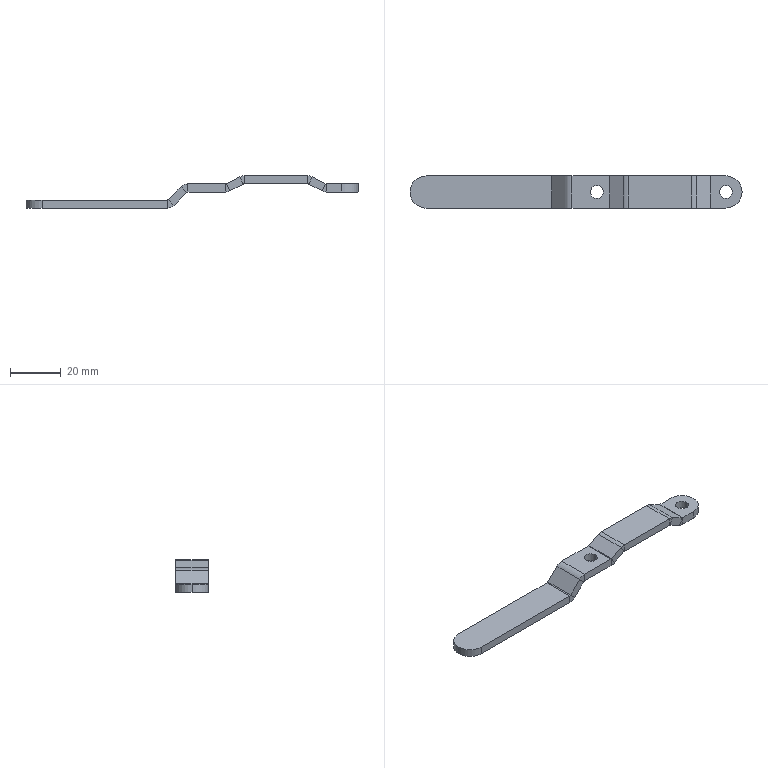Part | SolidWorks | features Fillet 3, Cut 1, Extrusion 1, FlattenBends 1, ProcessBends 1, SheetMetal 1 | 1 solid | 60 faces | box 130.683 x 12.7 x 12.7 mm | volume 5187 mm3 | plane 40 | cylinder 20 | commonest cylinder face diameters 1.27 x6 7.62 x6 5.08 x4 12.7 x4
STEP:
#1=CARTESIAN_POINT('',(-2.35,0.25,0.));
#2=VERTEX_POINT('',#1);
#3=CARTESIAN_POINT('',(-2.15,0.25,0.));
#4=VERTEX_POINT('',#3);
#5=CARTESIAN_POINT('',(-2.25,0.25,0.));
#6=DIRECTION('',(0.,0.,1.));
#7=DIRECTION('',(1.,0.,0.));
#8=AXIS2_PLACEMENT_3D('',#5,#6,#7);
#9=CIRCLE('',#8,0.1);
#10=EDGE_CURVE('',#2,#4,#9,.T.);
#11=ORIENTED_EDGE('',*,*,#10,.F.);
#12=CARTESIAN_POINT('',(-2.35,0.25,0.125));
#13=VERTEX_POINT('',#12);
#14=CARTESIAN_POINT('',(-2.35,0.25,-0.25));
#15=DIRECTION('',(0.,0.,1.));
#16=VECTOR('',#15,39.37);
#17=LINE('',#14,#16);
#18=EDGE_CURVE('',#2,#13,#17,.T.);
#19=ORIENTED_EDGE('',*,*,#18,.T.);
#20=CARTESIAN_POINT('',(-2.15,0.25,0.125));
#21=VERTEX_POINT('',#20);
#22=CARTESIAN_POINT('',(-2.25,0.25,0.125));
#23=DIRECTION('',(0.,0.,1.));
#24=DIRECTION('',(1.,0.,0.));
#25=AXIS2_PLACEMENT_3D('',#22,#23,#24);
#26=CIRCLE('',#25,0.1);
#27=EDGE_CURVE('',#13,#21,#26,.T.);
#28=ORIENTED_EDGE('',*,*,#27,.T.);
#29=CARTESIAN_POINT('',(-2.15,0.25,-0.25));
#30=DIRECTION('',(0.,0.,1.));
#31=VECTOR('',#30,39.37);
#32=LINE('',#29,#31);
#33=EDGE_CURVE('',#4,#21,#32,.T.);
#34=ORIENTED_EDGE('',*,*,#33,.F.);
#35=EDGE_LOOP('',(#11,#19,#28,#34));
#36=FACE_OUTER_BOUND('',#35,.T.);
#37=CARTESIAN_POINT('',(-2.25,0.25,-0.25));
#38=DIRECTION('',(0.,0.,1.));
#39=DIRECTION('',(1.,0.,0.));
#40=AXIS2_PLACEMENT_3D('',#37,#38,#39);
#41=CYLINDRICAL_SURFACE('',#40,0.1);
#42=ADVANCED_FACE('',(#36),#41,.F.);
#43=CARTESIAN_POINT('',(-0.35,0.25,0.));
#44=VERTEX_POINT('',#43);
#45=CARTESIAN_POINT('',(-0.15,0.25,0.));
#46=VERTEX_POINT('',#45);
#47=CARTESIAN_POINT('',(-0.25,0.25,0.));
#48=DIRECTION('',(0.,0.,1.));
#49=DIRECTION('',(1.,0.,0.));
#50=AXIS2_PLACEMENT_3D('',#47,#48,#49);
#51=CIRCLE('',#50,0.1);
#52=EDGE_CURVE('',#44,#46,#51,.T.);
#53=ORIENTED_EDGE('',*,*,#52,.F.);
#54=CARTESIAN_POINT('',(-0.35,0.25,0.125));
#55=VERTEX_POINT('',#54);
#56=CARTESIAN_POINT('',(-0.35,0.25,-0.25));
#57=DIRECTION('',(0.,0.,1.));
#58=VECTOR('',#57,39.37);
#59=LINE('',#56,#58);
#60=EDGE_CURVE('',#44,#55,#59,.T.);
#61=ORIENTED_EDGE('',*,*,#60,.T.);
#62=CARTESIAN_POINT('',(-0.15,0.25,0.125));
#63=VERTEX_POINT('',#62);
#64=CARTESIAN_POINT('',(-0.25,0.25,0.125));
#65=DIRECTION('',(0.,0.,1.));
#66=DIRECTION('',(1.,0.,0.));
#67=AXIS2_PLACEMENT_3D('',#64,#65,#66);
#68=CIRCLE('',#67,0.1);
#69=EDGE_CURVE('',#55,#63,#68,.T.);
#70=ORIENTED_EDGE('',*,*,#69,.T.);
#71=CARTESIAN_POINT('',(-0.15,0.25,-0.25));
#72=DIRECTION('',(0.,0.,1.));
#73=VECTOR('',#72,39.37);
#74=LINE('',#71,#73);
#75=EDGE_CURVE('',#46,#63,#74,.T.);
#76=ORIENTED_EDGE('',*,*,#75,.F.);
#77=EDGE_LOOP('',(#53,#61,#70,#76));
#78=FACE_OUTER_BOUND('',#77,.T.);
#79=CARTESIAN_POINT('',(-0.25,0.25,-0.25));
#80=DIRECTION('',(0.,0.,1.));
#81=DIRECTION('',(1.,0.,0.));
#82=AXIS2_PLACEMENT_3D('',#79,#80,#81);
#83=CYLINDRICAL_SURFACE('',#82,0.1);
#84=ADVANCED_FACE('',(#78),#83,.F.);
#85=CARTESIAN_POINT('',(-0.25,0.25,0.));
#86=DIRECTION('',(0.,0.,1.));
#87=DIRECTION('',(1.,0.,0.));
#88=AXIS2_PLACEMENT_3D('',#85,#86,#87);
#89=CIRCLE('',#88,0.1);
#90=EDGE_CURVE('',#46,#44,#89,.T.);
#91=ORIENTED_EDGE('',*,*,#90,.T.);
#92=ORIENTED_EDGE('',*,*,#52,.T.);
#93=EDGE_LOOP('',(#91,#92));
#94=FACE_BOUND('',#93,.T.);
#95=CARTESIAN_POINT('',(-0.25,0.5,0.));
#96=VERTEX_POINT('',#95);
#97=CARTESIAN_POINT('',(-0.4846,0.5,0.));
#98=VERTEX_POINT('',#97);
#99=CARTESIAN_POINT('',(0.,0.5,0.));
#100=DIRECTION('',(-1.,0.,0.));
#101=VECTOR('',#100,39.37);
#102=LINE('',#99,#101);
#103=EDGE_CURVE('',#96,#98,#102,.T.);
#104=ORIENTED_EDGE('',*,*,#103,.F.);
#105=CARTESIAN_POINT('',(0.,0.25,0.));
#106=VERTEX_POINT('',#105);
#107=CARTESIAN_POINT('',(-0.25,0.25,0.));
#108=DIRECTION('',(0.,0.,-1.));
#109=DIRECTION('',(1.,0.,0.));
#110=AXIS2_PLACEMENT_3D('',#107,#108,#109);
#111=CIRCLE('',#110,0.25);
#112=EDGE_CURVE('',#96,#106,#111,.T.);
#113=ORIENTED_EDGE('',*,*,#112,.T.);
#114=CARTESIAN_POINT('',(-0.25,0.,0.));
#115=VERTEX_POINT('',#114);
#116=CARTESIAN_POINT('',(-0.25,0.25,0.));
#117=DIRECTION('',(0.,0.,-1.));
#118=DIRECTION('',(1.,0.,0.));
#119=AXIS2_PLACEMENT_3D('',#116,#117,#118);
#120=CIRCLE('',#119,0.25);
#121=EDGE_CURVE('',#106,#115,#120,.T.);
#122=ORIENTED_EDGE('',*,*,#121,.T.);
#123=CARTESIAN_POINT('',(-0.4846,0.,0.));
#124=VERTEX_POINT('',#123);
#125=CARTESIAN_POINT('',(0.,0.,0.));
#126=DIRECTION('',(-1.,0.,0.));
#127=VECTOR('',#126,39.37);
#128=LINE('',#125,#127);
#129=EDGE_CURVE('',#115,#124,#128,.T.);
#130=ORIENTED_EDGE('',*,*,#129,.T.);
#131=CARTESIAN_POINT('',(-0.4846,0.5,0.));
#132=DIRECTION('',(0.,1.,0.));
#133=VECTOR('',#132,39.37);
#134=LINE('',#131,#133);
#135=EDGE_CURVE('',#124,#98,#134,.T.);
#136=ORIENTED_EDGE('',*,*,#135,.T.);
#137=EDGE_LOOP('',(#104,#113,#122,#130,#136));
#138=FACE_OUTER_BOUND('',#137,.T.);
#139=CARTESIAN_POINT('',(0.,0.5,0.));
#140=DIRECTION('',(0.,0.,1.));
#141=DIRECTION('',(1.,0.,0.));
#142=AXIS2_PLACEMENT_3D('',#139,#140,#141);
#143=PLANE('',#142);
#144=ADVANCED_FACE('',(#94,#138),#143,.F.);
#145=ORIENTED_EDGE('',*,*,#60,.F.);
#146=ORIENTED_EDGE('',*,*,#90,.F.);
#147=ORIENTED_EDGE('',*,*,#75,.T.);
#148=CARTESIAN_POINT('',(-0.25,0.25,0.125));
#149=DIRECTION('',(0.,0.,1.));
#150=DIRECTION('',(1.,0.,0.));
#151=AXIS2_PLACEMENT_3D('',#148,#149,#150);
#152=CIRCLE('',#151,0.1);
#153=EDGE_CURVE('',#63,#55,#152,.T.);
#154=ORIENTED_EDGE('',*,*,#153,.T.);
#155=EDGE_LOOP('',(#145,#146,#147,#154));
#156=FACE_OUTER_BOUND('',#155,.T.);
#157=CARTESIAN_POINT('',(-0.25,0.25,-0.25));
#158=DIRECTION('',(0.,0.,1.));
#159=DIRECTION('',(1.,0.,0.));
#160=AXIS2_PLACEMENT_3D('',#157,#158,#159);
#161=CYLINDRICAL_SURFACE('',#160,0.1);
#162=ADVANCED_FACE('',(#156),#161,.F.);
#163=ORIENTED_EDGE('',*,*,#153,.F.);
#164=ORIENTED_EDGE('',*,*,#69,.F.);
#165=EDGE_LOOP('',(#163,#164));
#166=FACE_BOUND('',#165,.T.);
#167=CARTESIAN_POINT('',(-0.25,0.,0.125));
#168=VERTEX_POINT('',#167);
#169=CARTESIAN_POINT('',(0.,0.25,0.125));
#170=VERTEX_POINT('',#169);
#171=CARTESIAN_POINT('',(-0.25,0.25,0.125));
#172=DIRECTION('',(0.,0.,1.));
#173=DIRECTION('',(1.,0.,0.));
#174=AXIS2_PLACEMENT_3D('',#171,#172,#173);
#175=CIRCLE('',#174,0.25);
#176=EDGE_CURVE('',#168,#170,#175,.T.);
#177=ORIENTED_EDGE('',*,*,#176,.T.);
#178=CARTESIAN_POINT('',(-0.25,0.5,0.125));
#179=VERTEX_POINT('',#178);
#180=CARTESIAN_POINT('',(-0.25,0.25,0.125));
#181=DIRECTION('',(0.,0.,1.));
#182=DIRECTION('',(1.,0.,0.));
#183=AXIS2_PLACEMENT_3D('',#180,#181,#182);
#184=CIRCLE('',#183,0.25);
#185=EDGE_CURVE('',#170,#179,#184,.T.);
#186=ORIENTED_EDGE('',*,*,#185,.T.);
#187=CARTESIAN_POINT('',(-0.4846,0.5,0.125));
#188=VERTEX_POINT('',#187);
#189=CARTESIAN_POINT('',(0.,0.5,0.125));
#190=DIRECTION('',(-1.,0.,0.));
#191=VECTOR('',#190,39.37);
#192=LINE('',#189,#191);
#193=EDGE_CURVE('',#179,#188,#192,.T.);
#194=ORIENTED_EDGE('',*,*,#193,.T.);
#195=CARTESIAN_POINT('',(-0.4846,0.,0.125));
#196=VERTEX_POINT('',#195);
#197=CARTESIAN_POINT('',(-0.4846,0.,0.125));
#198=DIRECTION('',(0.,-1.,0.));
#199=VECTOR('',#198,39.37);
#200=LINE('',#197,#199);
#201=EDGE_CURVE('',#188,#196,#200,.T.);
#202=ORIENTED_EDGE('',*,*,#201,.T.);
#203=CARTESIAN_POINT('',(0.,0.,0.125));
#204=DIRECTION('',(-1.,0.,0.));
#205=VECTOR('',#204,39.37);
#206=LINE('',#203,#205);
#207=EDGE_CURVE('',#168,#196,#206,.T.);
#208=ORIENTED_EDGE('',*,*,#207,.F.);
#209=EDGE_LOOP('',(#177,#186,#194,#202,#208));
#210=FACE_OUTER_BOUND('',#209,.T.);
#211=CARTESIAN_POINT('',(0.,0.5,0.125));
#212=DIRECTION('',(0.,0.,1.));
#213=DIRECTION('',(1.,0.,0.));
#214=AXIS2_PLACEMENT_3D('',#211,#212,#213);
#215=PLANE('',#214);
#216=ADVANCED_FACE('',(#166,#210),#215,.T.);
#217=CARTESIAN_POINT('',(-0.25,0.,1.518));
#218=DIRECTION('',(0.,0.,-1.));
#219=VECTOR('',#218,39.37);
#220=LINE('',#217,#219);
#221=EDGE_CURVE('',#168,#115,#220,.T.);
#222=ORIENTED_EDGE('',*,*,#221,.T.);
#223=ORIENTED_EDGE('',*,*,#121,.F.);
#224=CARTESIAN_POINT('',(0.,0.25,1.518));
#225=DIRECTION('',(0.,0.,-1.));
#226=VECTOR('',#225,39.37);
#227=LINE('',#224,#226);
#228=EDGE_CURVE('',#170,#106,#227,.T.);
#229=ORIENTED_EDGE('',*,*,#228,.F.);
#230=ORIENTED_EDGE('',*,*,#176,.F.);
#231=EDGE_LOOP('',(#222,#223,#229,#230));
#232=FACE_OUTER_BOUND('',#231,.T.);
#233=CARTESIAN_POINT('',(-0.25,0.25,1.518));
#234=DIRECTION('',(0.,0.,-1.));
#235=DIRECTION('',(-1.,0.,0.));
#236=AXIS2_PLACEMENT_3D('',#233,#234,#235);
#237=CYLINDRICAL_SURFACE('',#236,0.25);
#238=ADVANCED_FACE('',(#232),#237,.T.);
#239=ORIENTED_EDGE('',*,*,#228,.T.);
#240=ORIENTED_EDGE('',*,*,#112,.F.);
#241=CARTESIAN_POINT('',(-0.25,0.5,1.518));
#242=DIRECTION('',(0.,0.,-1.));
#243=VECTOR('',#242,39.37);
#244=LINE('',#241,#243);
#245=EDGE_CURVE('',#179,#96,#244,.T.);
#246=ORIENTED_EDGE('',*,*,#245,.F.);
#247=ORIENTED_EDGE('',*,*,#185,.F.);
#248=EDGE_LOOP('',(#239,#240,#246,#247));
#249=FACE_OUTER_BOUND('',#248,.T.);
#250=CARTESIAN_POINT('',(-0.25,0.25,1.518));
#251=DIRECTION('',(0.,0.,-1.));
#252=DIRECTION('',(-1.,0.,0.));
#253=AXIS2_PLACEMENT_3D('',#250,#251,#252);
#254=CYLINDRICAL_SURFACE('',#253,0.25);
#255=ADVANCED_FACE('',(#249),#254,.T.);
#256=ORIENTED_EDGE('',*,*,#245,.T.);
#257=ORIENTED_EDGE('',*,*,#103,.T.);
#258=CARTESIAN_POINT('',(-0.4846,0.5,1.518));
#259=DIRECTION('',(0.,0.,-1.));
#260=VECTOR('',#259,39.37);
#261=LINE('',#258,#260);
#262=EDGE_CURVE('',#188,#98,#261,.T.);
#263=ORIENTED_EDGE('',*,*,#262,.F.);
#264=ORIENTED_EDGE('',*,*,#193,.F.);
#265=EDGE_LOOP('',(#256,#257,#263,#264));
#266=FACE_OUTER_BOUND('',#265,.T.);
#267=CARTESIAN_POINT('',(0.,0.5,1.518));
#268=DIRECTION('',(0.,-1.,0.));
#269=DIRECTION('',(0.,0.,-1.));
#270=AXIS2_PLACEMENT_3D('',#267,#268,#269);
#271=PLANE('',#270);
#272=ADVANCED_FACE('',(#266),#271,.F.);
#273=ORIENTED_EDGE('',*,*,#129,.F.);
#274=ORIENTED_EDGE('',*,*,#221,.F.);
#275=ORIENTED_EDGE('',*,*,#207,.T.);
#276=CARTESIAN_POINT('',(-0.4846,0.,1.518));
#277=DIRECTION('',(0.,0.,-1.));
#278=VECTOR('',#277,39.37);
#279=LINE('',#276,#278);
#280=EDGE_CURVE('',#196,#124,#279,.T.);
#281=ORIENTED_EDGE('',*,*,#280,.T.);
#282=EDGE_LOOP('',(#273,#274,#275,#281));
#283=FACE_OUTER_BOUND('',#282,.T.);
#284=CARTESIAN_POINT('',(0.,0.,1.518));
#285=DIRECTION('',(0.,-1.,0.));
#286=DIRECTION('',(0.,0.,-1.));
#287=AXIS2_PLACEMENT_3D('',#284,#285,#286);
#288=PLANE('',#287);
#289=ADVANCED_FACE('',(#283),#288,.T.);
#290=CARTESIAN_POINT('',(-0.7647,0.5,0.1224));
#291=VERTEX_POINT('',#290);
#292=CARTESIAN_POINT('',(-0.7088,0.5,0.2342));
#293=VERTEX_POINT('',#292);
#294=CARTESIAN_POINT('',(-1.204,0.5,-0.7566));
#295=DIRECTION('',(0.4472,0.,0.8944));
#296=VECTOR('',#295,39.37);
#297=LINE('',#294,#296);
#298=EDGE_CURVE('',#291,#293,#297,.T.);
#299=ORIENTED_EDGE('',*,*,#298,.T.);
#300=CARTESIAN_POINT('',(-0.4958,0.5,0.1276));
#301=VERTEX_POINT('',#300);
#302=CARTESIAN_POINT('',(-0.4905,0.5,0.125));
#303=DIRECTION('',(-0.8944,0.,0.4472));
#304=VECTOR('',#303,39.37);
#305=LINE('',#302,#304);
#306=EDGE_CURVE('',#301,#293,#305,.T.);
#307=ORIENTED_EDGE('',*,*,#306,.F.);
#308=CARTESIAN_POINT('',(-0.5517,0.5,0.01584));
#309=VERTEX_POINT('',#308);
#310=CARTESIAN_POINT('',(-0.9911,0.5,-0.8631));
#311=DIRECTION('',(0.4472,0.,0.8944));
#312=VECTOR('',#311,39.37);
#313=LINE('',#310,#312);
#314=EDGE_CURVE('',#309,#301,#313,.T.);
#315=ORIENTED_EDGE('',*,*,#314,.F.);
#316=CARTESIAN_POINT('',(-0.52,0.5,0.));
#317=DIRECTION('',(-0.8944,0.,0.4472));
#318=VECTOR('',#317,39.37);
#319=LINE('',#316,#318);
#320=EDGE_CURVE('',#309,#291,#319,.T.);
#321=ORIENTED_EDGE('',*,*,#320,.T.);
#322=EDGE_LOOP('',(#299,#307,#315,#321));
#323=FACE_OUTER_BOUND('',#322,.T.);
#324=CARTESIAN_POINT('',(-0.9595,0.5,-0.8789));
#325=DIRECTION('',(0.,1.,0.));
#326=DIRECTION('',(0.4472,0.,0.8944));
#327=AXIS2_PLACEMENT_3D('',#324,#325,#326);
#328=PLANE('',#327);
#329=ADVANCED_FACE('',(#323),#328,.T.);
#330=CARTESIAN_POINT('',(-0.4958,0.,0.1276));
#331=VERTEX_POINT('',#330);
#332=CARTESIAN_POINT('',(-0.7088,0.,0.2342));
#333=VERTEX_POINT('',#332);
#334=CARTESIAN_POINT('',(-0.4905,0.,0.125));
#335=DIRECTION('',(-0.8944,0.,0.4472));
#336=VECTOR('',#335,39.37);
#337=LINE('',#334,#336);
#338=EDGE_CURVE('',#331,#333,#337,.T.);
#339=ORIENTED_EDGE('',*,*,#338,.T.);
#340=CARTESIAN_POINT('',(-0.7647,0.,0.1224));
#341=VERTEX_POINT('',#340);
#342=CARTESIAN_POINT('',(-1.204,0.,-0.7566));
#343=DIRECTION('',(0.4472,0.,0.8944));
#344=VECTOR('',#343,39.37);
#345=LINE('',#342,#344);
#346=EDGE_CURVE('',#341,#333,#345,.T.);
#347=ORIENTED_EDGE('',*,*,#346,.F.);
#348=CARTESIAN_POINT('',(-0.5517,0.,0.01584));
#349=VERTEX_POINT('',#348);
#350=CARTESIAN_POINT('',(-0.52,0.,0.));
#351=DIRECTION('',(-0.8944,0.,0.4472));
#352=VECTOR('',#351,39.37);
#353=LINE('',#350,#352);
#354=EDGE_CURVE('',#349,#341,#353,.T.);
#355=ORIENTED_EDGE('',*,*,#354,.F.);
#356=CARTESIAN_POINT('',(-0.9911,0.,-0.8631));
#357=DIRECTION('',(0.4472,0.,0.8944));
#358=VECTOR('',#357,39.37);
#359=LINE('',#356,#358);
#360=EDGE_CURVE('',#349,#331,#359,.T.);
#361=ORIENTED_EDGE('',*,*,#360,.T.);
#362=EDGE_LOOP('',(#339,#347,#355,#361));
#363=FACE_OUTER_BOUND('',#362,.T.);
#364=CARTESIAN_POINT('',(-0.9595,0.,-0.8789));
#365=DIRECTION('',(0.,1.,0.));
#366=DIRECTION('',(0.4472,0.,0.8944));
#367=AXIS2_PLACEMENT_3D('',#364,#365,#366);
#368=PLANE('',#367);
#369=ADVANCED_FACE('',(#363),#368,.F.);
#370=ORIENTED_EDGE('',*,*,#320,.F.);
#371=CARTESIAN_POINT('',(-0.5517,0.5,0.01584));
#372=DIRECTION('',(0.,-1.,0.));
#373=VECTOR('',#372,39.37);
#374=LINE('',#371,#373);
#375=EDGE_CURVE('',#309,#349,#374,.T.);
#376=ORIENTED_EDGE('',*,*,#375,.T.);
#377=ORIENTED_EDGE('',*,*,#354,.T.);
#378=CARTESIAN_POINT('',(-0.7647,0.5,0.1224));
#379=DIRECTION('',(0.,1.,0.));
#380=VECTOR('',#379,39.37);
#381=LINE('',#378,#380);
#382=EDGE_CURVE('',#341,#291,#381,.T.);
#383=ORIENTED_EDGE('',*,*,#382,.T.);
#384=EDGE_LOOP('',(#370,#376,#377,#383));
#385=FACE_OUTER_BOUND('',#384,.T.);
#386=CARTESIAN_POINT('',(-0.52,0.5,0.));
#387=DIRECTION('',(0.4472,0.,0.8944));
#388=DIRECTION('',(0.8944,0.,-0.4472));
#389=AXIS2_PLACEMENT_3D('',#386,#387,#388);
#390=PLANE('',#389);
#391=ADVANCED_FACE('',(#385),#390,.F.);
#392=ORIENTED_EDGE('',*,*,#306,.T.);
#393=CARTESIAN_POINT('',(-0.7088,0.5,0.2342));
#394=DIRECTION('',(0.,-1.,0.));
#395=VECTOR('',#394,39.37);
#396=LINE('',#393,#395);
#397=EDGE_CURVE('',#293,#333,#396,.T.);
#398=ORIENTED_EDGE('',*,*,#397,.T.);
#399=ORIENTED_EDGE('',*,*,#338,.F.);
#400=CARTESIAN_POINT('',(-0.4958,0.5,0.1276));
#401=DIRECTION('',(0.,1.,0.));
#402=VECTOR('',#401,39.37);
#403=LINE('',#400,#402);
#404=EDGE_CURVE('',#331,#301,#403,.T.);
#405=ORIENTED_EDGE('',*,*,#404,.T.);
#406=EDGE_LOOP('',(#392,#398,#399,#405));
#407=FACE_OUTER_BOUND('',#406,.T.);
#408=CARTESIAN_POINT('',(-0.4905,0.5,0.125));
#409=DIRECTION('',(0.4472,0.,0.8944));
#410=DIRECTION('',(0.8944,0.,-0.4472));
#411=AXIS2_PLACEMENT_3D('',#408,#409,#410);
#412=PLANE('',#411);
#413=ADVANCED_FACE('',(#407),#412,.T.);
#414=CARTESIAN_POINT('',(-0.7759,0.,0.25));
#415=VERTEX_POINT('',#414);
#416=CARTESIAN_POINT('',(-1.764,0.,0.25));
#417=VERTEX_POINT('',#416);
#418=CARTESIAN_POINT('',(-0.7405,0.,0.25));
#419=DIRECTION('',(-1.,0.,0.));
#420=VECTOR('',#419,39.37);
#421=LINE('',#418,#420);
#422=EDGE_CURVE('',#415,#417,#421,.T.);
#423=ORIENTED_EDGE('',*,*,#422,.T.);
#424=CARTESIAN_POINT('',(-1.764,0.,0.125));
#425=VERTEX_POINT('',#424);
#426=CARTESIAN_POINT('',(-1.764,0.,-1.965));
#427=DIRECTION('',(0.,0.,1.));
#428=VECTOR('',#427,39.37);
#429=LINE('',#426,#428);
#430=EDGE_CURVE('',#425,#417,#429,.T.);
#431=ORIENTED_EDGE('',*,*,#430,.F.);
#432=CARTESIAN_POINT('',(-0.7759,0.,0.125));
#433=VERTEX_POINT('',#432);
#434=CARTESIAN_POINT('',(-0.77,0.,0.125));
#435=DIRECTION('',(-1.,0.,0.));
#436=VECTOR('',#435,39.37);
#437=LINE('',#434,#436);
#438=EDGE_CURVE('',#433,#425,#437,.T.);
#439=ORIENTED_EDGE('',*,*,#438,.F.);
#440=CARTESIAN_POINT('',(-0.7759,0.,-1.965));
#441=DIRECTION('',(0.,0.,1.));
#442=VECTOR('',#441,39.37);
#443=LINE('',#440,#442);
#444=EDGE_CURVE('',#433,#415,#443,.T.);
#445=ORIENTED_EDGE('',*,*,#444,.T.);
#446=EDGE_LOOP('',(#423,#431,#439,#445));
#447=FACE_OUTER_BOUND('',#446,.T.);
#448=CARTESIAN_POINT('',(-0.77,0.,-1.965));
#449=DIRECTION('',(0.,1.,0.));
#450=DIRECTION('',(0.,0.,1.));
#451=AXIS2_PLACEMENT_3D('',#448,#449,#450);
#452=PLANE('',#451);
#453=ADVANCED_FACE('',(#447),#452,.F.);
#454=CARTESIAN_POINT('',(-1.764,0.5,0.125));
#455=VERTEX_POINT('',#454);
#456=CARTESIAN_POINT('',(-1.764,0.5,0.25));
#457=VERTEX_POINT('',#456);
#458=CARTESIAN_POINT('',(-1.764,0.5,-1.965));
#459=DIRECTION('',(0.,0.,1.));
#460=VECTOR('',#459,39.37);
#461=LINE('',#458,#460);
#462=EDGE_CURVE('',#455,#457,#461,.T.);
#463=ORIENTED_EDGE('',*,*,#462,.T.);
#464=CARTESIAN_POINT('',(-0.7759,0.5,0.25));
#465=VERTEX_POINT('',#464);
#466=CARTESIAN_POINT('',(-0.7405,0.5,0.25));
#467=DIRECTION('',(-1.,0.,0.));
#468=VECTOR('',#467,39.37);
#469=LINE('',#466,#468);
#470=EDGE_CURVE('',#465,#457,#469,.T.);
#471=ORIENTED_EDGE('',*,*,#470,.F.);
#472=CARTESIAN_POINT('',(-0.7759,0.5,0.125));
#473=VERTEX_POINT('',#472);
#474=CARTESIAN_POINT('',(-0.7759,0.5,-1.965));
#475=DIRECTION('',(0.,0.,1.));
#476=VECTOR('',#475,39.37);
#477=LINE('',#474,#476);
#478=EDGE_CURVE('',#473,#465,#477,.T.);
#479=ORIENTED_EDGE('',*,*,#478,.F.);
#480=CARTESIAN_POINT('',(-0.77,0.5,0.125));
#481=DIRECTION('',(-1.,0.,0.));
#482=VECTOR('',#481,39.37);
#483=LINE('',#480,#482);
#484=EDGE_CURVE('',#473,#455,#483,.T.);
#485=ORIENTED_EDGE('',*,*,#484,.T.);
#486=EDGE_LOOP('',(#463,#471,#479,#485));
#487=FACE_OUTER_BOUND('',#486,.T.);
#488=CARTESIAN_POINT('',(-0.77,0.5,-1.965));
#489=DIRECTION('',(0.,1.,0.));
#490=DIRECTION('',(0.,0.,1.));
#491=AXIS2_PLACEMENT_3D('',#488,#489,#490);
#492=PLANE('',#491);
#493=ADVANCED_FACE('',(#487),#492,.T.);
#494=ORIENTED_EDGE('',*,*,#438,.T.);
#495=CARTESIAN_POINT('',(-1.764,0.5,0.125));
#496=DIRECTION('',(0.,1.,0.));
#497=VECTOR('',#496,39.37);
#498=LINE('',#495,#497);
#499=EDGE_CURVE('',#425,#455,#498,.T.);
#500=ORIENTED_EDGE('',*,*,#499,.T.);
#501=ORIENTED_EDGE('',*,*,#484,.F.);
#502=CARTESIAN_POINT('',(-0.7759,0.,0.125));
#503=DIRECTION('',(0.,-1.,0.));
#504=VECTOR('',#503,39.37);
#505=LINE('',#502,#504);
#506=EDGE_CURVE('',#473,#433,#505,.T.);
#507=ORIENTED_EDGE('',*,*,#506,.T.);
#508=EDGE_LOOP('',(#494,#500,#501,#507));
#509=FACE_OUTER_BOUND('',#508,.T.);
#510=CARTESIAN_POINT('',(-0.77,0.5,0.125));
#511=DIRECTION('',(0.,0.,1.));
#512=DIRECTION('',(1.,0.,0.));
#513=AXIS2_PLACEMENT_3D('',#510,#511,#512);
#514=PLANE('',#513);
#515=ADVANCED_FACE('',(#509),#514,.F.);
#516=ORIENTED_EDGE('',*,*,#470,.T.);
#517=CARTESIAN_POINT('',(-1.764,0.5,0.25));
#518=DIRECTION('',(0.,-1.,0.));
#519=VECTOR('',#518,39.37);
#520=LINE('',#517,#519);
#521=EDGE_CURVE('',#457,#417,#520,.T.);
#522=ORIENTED_EDGE('',*,*,#521,.T.);
#523=ORIENTED_EDGE('',*,*,#422,.F.);
#524=CARTESIAN_POINT('',(-0.7759,0.5,0.25));
#525=DIRECTION('',(0.,1.,0.));
#526=VECTOR('',#525,39.37);
#527=LINE('',#524,#526);
#528=EDGE_CURVE('',#415,#465,#527,.T.);
#529=ORIENTED_EDGE('',*,*,#528,.T.);
#530=EDGE_LOOP('',(#516,#522,#523,#529));
#531=FACE_OUTER_BOUND('',#530,.T.);
#532=CARTESIAN_POINT('',(-0.7405,0.5,0.25));
#533=DIRECTION('',(0.,0.,1.));
#534=DIRECTION('',(1.,0.,0.));
#535=AXIS2_PLACEMENT_3D('',#532,#533,#534);
#536=PLANE('',#535);
#537=ADVANCED_FACE('',(#531),#536,.T.);
#538=CARTESIAN_POINT('',(-1.775,0.,0.1224));
#539=VERTEX_POINT('',#538);
#540=CARTESIAN_POINT('',(-1.988,0.,0.01584));
#541=VERTEX_POINT('',#540);
#542=CARTESIAN_POINT('',(-1.77,0.,0.125));
#543=DIRECTION('',(-0.8944,0.,-0.4472));
#544=VECTOR('',#543,39.37);
#545=LINE('',#542,#544);
#546=EDGE_CURVE('',#539,#541,#545,.T.);
#547=ORIENTED_EDGE('',*,*,#546,.T.);
#548=CARTESIAN_POINT('',(-1.988,0.5,0.01584));
#549=VERTEX_POINT('',#548);
#550=CARTESIAN_POINT('',(-1.988,0.5,0.01584));
#551=DIRECTION('',(0.,1.,0.));
#552=VECTOR('',#551,39.37);
#553=LINE('',#550,#552);
#554=EDGE_CURVE('',#541,#549,#553,.T.);
#555=ORIENTED_EDGE('',*,*,#554,.T.);
#556=CARTESIAN_POINT('',(-1.775,0.5,0.1224));
#557=VERTEX_POINT('',#556);
#558=CARTESIAN_POINT('',(-1.77,0.5,0.125));
#559=DIRECTION('',(-0.8944,0.,-0.4472));
#560=VECTOR('',#559,39.37);
#561=LINE('',#558,#560);
#562=EDGE_CURVE('',#557,#549,#561,.T.);
#563=ORIENTED_EDGE('',*,*,#562,.F.);
#564=CARTESIAN_POINT('',(-1.775,0.,0.1224));
#565=DIRECTION('',(0.,-1.,0.));
#566=VECTOR('',#565,39.37);
#567=LINE('',#564,#566);
#568=EDGE_CURVE('',#557,#539,#567,.T.);
#569=ORIENTED_EDGE('',*,*,#568,.T.);
#570=EDGE_LOOP('',(#547,#555,#563,#569));
#571=FACE_OUTER_BOUND('',#570,.T.);
#572=CARTESIAN_POINT('',(-1.77,0.5,0.125));
#573=DIRECTION('',(-0.4472,0.,0.8944));
#574=DIRECTION('',(0.8944,0.,0.4472));
#575=AXIS2_PLACEMENT_3D('',#572,#573,#574);
#576=PLANE('',#575);
#577=ADVANCED_FACE('',(#571),#576,.F.);
#578=ORIENTED_EDGE('',*,*,#546,.F.);
#579=CARTESIAN_POINT('',(-1.831,0.,0.2342));
#580=VERTEX_POINT('',#579);
#581=CARTESIAN_POINT('',(-2.327,0.,1.225));
#582=DIRECTION('',(0.4472,0.,-0.8944));
#583=VECTOR('',#582,39.37);
#584=LINE('',#581,#583);
#585=EDGE_CURVE('',#580,#539,#584,.T.);
#586=ORIENTED_EDGE('',*,*,#585,.F.);
#587=CARTESIAN_POINT('',(-2.044,0.,0.1276));
#588=VERTEX_POINT('',#587);
#589=CARTESIAN_POINT('',(-1.8,0.,0.25));
#590=DIRECTION('',(-0.8944,0.,-0.4472));
#591=VECTOR('',#590,39.37);
#592=LINE('',#589,#591);
#593=EDGE_CURVE('',#580,#588,#592,.T.);
#594=ORIENTED_EDGE('',*,*,#593,.T.);
#595=CARTESIAN_POINT('',(-2.54,0.,1.118));
#596=DIRECTION('',(0.4472,0.,-0.8944));
#597=VECTOR('',#596,39.37);
#598=LINE('',#595,#597);
#599=EDGE_CURVE('',#588,#541,#598,.T.);
#600=ORIENTED_EDGE('',*,*,#599,.T.);
#601=EDGE_LOOP('',(#578,#586,#594,#600));
#602=FACE_OUTER_BOUND('',#601,.T.);
#603=CARTESIAN_POINT('',(-2.295,0.,1.241));
#604=DIRECTION('',(0.,-1.,0.));
#605=DIRECTION('',(0.4472,0.,-0.8944));
#606=AXIS2_PLACEMENT_3D('',#603,#604,#605);
#607=PLANE('',#606);
#608=ADVANCED_FACE('',(#602),#607,.T.);
#609=CARTESIAN_POINT('',(-1.831,0.5,0.2342));
#610=VERTEX_POINT('',#609);
#611=CARTESIAN_POINT('',(-2.327,0.5,1.225));
#612=DIRECTION('',(0.4472,0.,-0.8944));
#613=VECTOR('',#612,39.37);
#614=LINE('',#611,#613);
#615=EDGE_CURVE('',#610,#557,#614,.T.);
#616=ORIENTED_EDGE('',*,*,#615,.T.);
#617=ORIENTED_EDGE('',*,*,#562,.T.);
#618=CARTESIAN_POINT('',(-2.044,0.5,0.1276));
#619=VERTEX_POINT('',#618);
#620=CARTESIAN_POINT('',(-2.54,0.5,1.118));
#621=DIRECTION('',(0.4472,0.,-0.8944));
#622=VECTOR('',#621,39.37);
#623=LINE('',#620,#622);
#624=EDGE_CURVE('',#619,#549,#623,.T.);
#625=ORIENTED_EDGE('',*,*,#624,.F.);
#626=CARTESIAN_POINT('',(-1.8,0.5,0.25));
#627=DIRECTION('',(-0.8944,0.,-0.4472));
#628=VECTOR('',#627,39.37);
#629=LINE('',#626,#628);
#630=EDGE_CURVE('',#610,#619,#629,.T.);
#631=ORIENTED_EDGE('',*,*,#630,.F.);
#632=EDGE_LOOP('',(#616,#617,#625,#631));
#633=FACE_OUTER_BOUND('',#632,.T.);
#634=CARTESIAN_POINT('',(-2.295,0.5,1.241));
#635=DIRECTION('',(0.,-1.,0.));
#636=DIRECTION('',(0.4472,0.,-0.8944));
#637=AXIS2_PLACEMENT_3D('',#634,#635,#636);
#638=PLANE('',#637);
#639=ADVANCED_FACE('',(#633),#638,.F.);
#640=ORIENTED_EDGE('',*,*,#593,.F.);
#641=CARTESIAN_POINT('',(-1.831,0.5,0.2342));
#642=DIRECTION('',(0.,1.,0.));
#643=VECTOR('',#642,39.37);
#644=LINE('',#641,#643);
#645=EDGE_CURVE('',#580,#610,#644,.T.);
#646=ORIENTED_EDGE('',*,*,#645,.T.);
#647=ORIENTED_EDGE('',*,*,#630,.T.);
#648=CARTESIAN_POINT('',(-2.044,0.,0.1276));
#649=DIRECTION('',(0.,-1.,0.));
#650=VECTOR('',#649,39.37);
#651=LINE('',#648,#650);
#652=EDGE_CURVE('',#619,#588,#651,.T.);
#653=ORIENTED_EDGE('',*,*,#652,.T.);
#654=EDGE_LOOP('',(#640,#646,#647,#653));
#655=FACE_OUTER_BOUND('',#654,.T.);
#656=CARTESIAN_POINT('',(-1.8,0.5,0.25));
#657=DIRECTION('',(-0.4472,0.,0.8944));
#658=DIRECTION('',(0.8944,0.,0.4472));
#659=AXIS2_PLACEMENT_3D('',#656,#657,#658);
#660=PLANE('',#659);
#661=ADVANCED_FACE('',(#655),#660,.T.);
#662=CARTESIAN_POINT('',(-2.25,0.25,0.125));
#663=DIRECTION('',(0.,0.,1.));
#664=DIRECTION('',(1.,0.,0.));
#665=AXIS2_PLACEMENT_3D('',#662,#663,#664);
#666=CIRCLE('',#665,0.1);
#667=EDGE_CURVE('',#21,#13,#666,.T.);
#668=ORIENTED_EDGE('',*,*,#667,.F.);
#669=ORIENTED_EDGE('',*,*,#27,.F.);
#670=EDGE_LOOP('',(#668,#669));
#671=FACE_BOUND('',#670,.T.);
#672=CARTESIAN_POINT('',(-2.055,0.5,0.125));
#673=VERTEX_POINT('',#672);
#674=CARTESIAN_POINT('',(-2.635,0.5,0.125));
#675=VERTEX_POINT('',#674);
#676=CARTESIAN_POINT('',(-2.05,0.5,0.125));
#677=DIRECTION('',(-1.,0.,0.));
#678=VECTOR('',#677,39.37);
#679=LINE('',#676,#678);
#680=EDGE_CURVE('',#673,#675,#679,.T.);
#681=ORIENTED_EDGE('',*,*,#680,.T.);
#682=CARTESIAN_POINT('',(-2.635,0.,0.125));
#683=VERTEX_POINT('',#682);
#684=CARTESIAN_POINT('',(-2.635,0.5,0.125));
#685=DIRECTION('',(0.,-1.,0.));
#686=VECTOR('',#685,39.37);
#687=LINE('',#684,#686);
#688=EDGE_CURVE('',#675,#683,#687,.T.);
#689=ORIENTED_EDGE('',*,*,#688,.T.);
#690=CARTESIAN_POINT('',(-2.055,0.,0.125));
#691=VERTEX_POINT('',#690);
#692=CARTESIAN_POINT('',(-2.05,0.,0.125));
#693=DIRECTION('',(-1.,0.,0.));
#694=VECTOR('',#693,39.37);
#695=LINE('',#692,#694);
#696=EDGE_CURVE('',#691,#683,#695,.T.);
#697=ORIENTED_EDGE('',*,*,#696,.F.);
#698=CARTESIAN_POINT('',(-2.055,0.5,0.125));
#699=DIRECTION('',(0.,1.,0.));
#700=VECTOR('',#699,39.37);
#701=LINE('',#698,#700);
#702=EDGE_CURVE('',#691,#673,#701,.T.);
#703=ORIENTED_EDGE('',*,*,#702,.T.);
#704=EDGE_LOOP('',(#681,#689,#697,#703));
#705=FACE_OUTER_BOUND('',#704,.T.);
#706=CARTESIAN_POINT('',(-2.05,0.5,0.125));
#707=DIRECTION('',(0.,0.,1.));
#708=DIRECTION('',(1.,0.,0.));
#709=AXIS2_PLACEMENT_3D('',#706,#707,#708);
#710=PLANE('',#709);
#711=ADVANCED_FACE('',(#671,#705),#710,.T.);
#712=ORIENTED_EDGE('',*,*,#18,.F.);
#713=CARTESIAN_POINT('',(-2.25,0.25,0.));
#714=DIRECTION('',(0.,0.,1.));
#715=DIRECTION('',(1.,0.,0.));
#716=AXIS2_PLACEMENT_3D('',#713,#714,#715);
#717=CIRCLE('',#716,0.1);
#718=EDGE_CURVE('',#4,#2,#717,.T.);
#719=ORIENTED_EDGE('',*,*,#718,.F.);
#720=ORIENTED_EDGE('',*,*,#33,.T.);
#721=ORIENTED_EDGE('',*,*,#667,.T.);
#722=EDGE_LOOP('',(#712,#719,#720,#721));
#723=FACE_OUTER_BOUND('',#722,.T.);
#724=CARTESIAN_POINT('',(-2.25,0.25,-0.25));
#725=DIRECTION('',(0.,0.,1.));
#726=DIRECTION('',(1.,0.,0.));
#727=AXIS2_PLACEMENT_3D('',#724,#725,#726);
#728=CYLINDRICAL_SURFACE('',#727,0.1);
#729=ADVANCED_FACE('',(#723),#728,.F.);
#730=ORIENTED_EDGE('',*,*,#718,.T.);
#731=ORIENTED_EDGE('',*,*,#10,.T.);
#732=EDGE_LOOP('',(#730,#731));
#733=FACE_BOUND('',#732,.T.);
#734=CARTESIAN_POINT('',(-2.055,0.5,0.));
#735=VERTEX_POINT('',#734);
#736=CARTESIAN_POINT('',(-2.635,0.5,0.));
#737=VERTEX_POINT('',#736);
#738=CARTESIAN_POINT('',(-2.02,0.5,0.));
#739=DIRECTION('',(-1.,0.,0.));
#740=VECTOR('',#739,39.37);
#741=LINE('',#738,#740);
#742=EDGE_CURVE('',#735,#737,#741,.T.);
#743=ORIENTED_EDGE('',*,*,#742,.F.);
#744=CARTESIAN_POINT('',(-2.055,0.,0.));
#745=VERTEX_POINT('',#744);
#746=CARTESIAN_POINT('',(-2.055,0.5,0.));
#747=DIRECTION('',(0.,-1.,0.));
#748=VECTOR('',#747,39.37);
#749=LINE('',#746,#748);
#750=EDGE_CURVE('',#735,#745,#749,.T.);
#751=ORIENTED_EDGE('',*,*,#750,.T.);
#752=CARTESIAN_POINT('',(-2.635,0.,0.));
#753=VERTEX_POINT('',#752);
#754=CARTESIAN_POINT('',(-2.02,0.,0.));
#755=DIRECTION('',(-1.,0.,0.));
#756=VECTOR('',#755,39.37);
#757=LINE('',#754,#756);
#758=EDGE_CURVE('',#745,#753,#757,.T.);
#759=ORIENTED_EDGE('',*,*,#758,.T.);
#760=CARTESIAN_POINT('',(-2.635,0.5,0.));
#761=DIRECTION('',(0.,1.,0.));
#762=VECTOR('',#761,39.37);
#763=LINE('',#760,#762);
#764=EDGE_CURVE('',#753,#737,#763,.T.);
#765=ORIENTED_EDGE('',*,*,#764,.T.);
#766=EDGE_LOOP('',(#743,#751,#759,#765));
#767=FACE_OUTER_BOUND('',#766,.T.);
#768=CARTESIAN_POINT('',(-2.02,0.5,0.));
#769=DIRECTION('',(0.,0.,1.));
#770=DIRECTION('',(1.,0.,0.));
#771=AXIS2_PLACEMENT_3D('',#768,#769,#770);
#772=PLANE('',#771);
#773=ADVANCED_FACE('',(#733,#767),#772,.F.);
#774=CARTESIAN_POINT('',(-2.635,0.5,-1.405));
#775=DIRECTION('',(0.,0.,1.));
#776=VECTOR('',#775,39.37);
#777=LINE('',#774,#776);
#778=EDGE_CURVE('',#737,#675,#777,.T.);
#779=ORIENTED_EDGE('',*,*,#778,.T.);
#780=ORIENTED_EDGE('',*,*,#680,.F.);
#781=CARTESIAN_POINT('',(-2.055,0.5,-1.405));
#782=DIRECTION('',(0.,0.,1.));
#783=VECTOR('',#782,39.37);
#784=LINE('',#781,#783);
#785=EDGE_CURVE('',#735,#673,#784,.T.);
#786=ORIENTED_EDGE('',*,*,#785,.F.);
#787=ORIENTED_EDGE('',*,*,#742,.T.);
#788=EDGE_LOOP('',(#779,#780,#786,#787));
#789=FACE_OUTER_BOUND('',#788,.T.);
#790=CARTESIAN_POINT('',(-2.02,0.5,-1.405));
#791=DIRECTION('',(0.,1.,0.));
#792=DIRECTION('',(0.,0.,1.));
#793=AXIS2_PLACEMENT_3D('',#790,#791,#792);
#794=PLANE('',#793);
#795=ADVANCED_FACE('',(#789),#794,.T.);
#796=ORIENTED_EDGE('',*,*,#696,.T.);
#797=CARTESIAN_POINT('',(-2.635,0.,-1.405));
#798=DIRECTION('',(0.,0.,1.));
#799=VECTOR('',#798,39.37);
#800=LINE('',#797,#799);
#801=EDGE_CURVE('',#753,#683,#800,.T.);
#802=ORIENTED_EDGE('',*,*,#801,.F.);
#803=ORIENTED_EDGE('',*,*,#758,.F.);
#804=CARTESIAN_POINT('',(-2.055,0.,-1.405));
#805=DIRECTION('',(0.,0.,1.));
#806=VECTOR('',#805,39.37);
#807=LINE('',#804,#806);
#808=EDGE_CURVE('',#745,#691,#807,.T.);
#809=ORIENTED_EDGE('',*,*,#808,.T.);
#810=EDGE_LOOP('',(#796,#802,#803,#809));
#811=FACE_OUTER_BOUND('',#810,.T.);
#812=CARTESIAN_POINT('',(-2.02,0.,-1.405));
#813=DIRECTION('',(0.,1.,0.));
#814=DIRECTION('',(0.,0.,1.));
#815=AXIS2_PLACEMENT_3D('',#812,#813,#814);
#816=PLANE('',#815);
#817=ADVANCED_FACE('',(#811),#816,.F.);
#818=CARTESIAN_POINT('',(-2.652,0.,-0.007322));
#819=VERTEX_POINT('',#818);
#820=CARTESIAN_POINT('',(-2.851,0.,-0.2061));
#821=VERTEX_POINT('',#820);
#822=CARTESIAN_POINT('',(-2.645,0.,0.));
#823=DIRECTION('',(-0.7071,0.,-0.7071));
#824=VECTOR('',#823,39.37);
#825=LINE('',#822,#824);
#826=EDGE_CURVE('',#819,#821,#825,.T.);
#827=ORIENTED_EDGE('',*,*,#826,.T.);
#828=CARTESIAN_POINT('',(-2.851,0.5,-0.2061));
#829=VERTEX_POINT('',#828);
#830=CARTESIAN_POINT('',(-2.851,0.5,-0.2061));
#831=DIRECTION('',(0.,1.,0.));
#832=VECTOR('',#831,39.37);
#833=LINE('',#830,#832);
#834=EDGE_CURVE('',#821,#829,#833,.T.);
#835=ORIENTED_EDGE('',*,*,#834,.T.);
#836=CARTESIAN_POINT('',(-2.652,0.5,-0.007322));
#837=VERTEX_POINT('',#836);
#838=CARTESIAN_POINT('',(-2.645,0.5,0.));
#839=DIRECTION('',(-0.7071,0.,-0.7071));
#840=VECTOR('',#839,39.37);
#841=LINE('',#838,#840);
#842=EDGE_CURVE('',#837,#829,#841,.T.);
#843=ORIENTED_EDGE('',*,*,#842,.F.);
#844=CARTESIAN_POINT('',(-2.652,0.,-0.007322));
#845=DIRECTION('',(0.,-1.,0.));
#846=VECTOR('',#845,39.37);
#847=LINE('',#844,#846);
#848=EDGE_CURVE('',#837,#819,#847,.T.);
#849=ORIENTED_EDGE('',*,*,#848,.T.);
#850=EDGE_LOOP('',(#827,#835,#843,#849));
#851=FACE_OUTER_BOUND('',#850,.T.);
#852=CARTESIAN_POINT('',(-2.645,0.5,0.));
#853=DIRECTION('',(-0.7071,0.,0.7071));
#854=DIRECTION('',(0.7071,0.,0.7071));
#855=AXIS2_PLACEMENT_3D('',#852,#853,#854);
#856=PLANE('',#855);
#857=ADVANCED_FACE('',(#851),#856,.F.);
#858=ORIENTED_EDGE('',*,*,#826,.F.);
#859=CARTESIAN_POINT('',(-2.741,0.,0.08107));
#860=VERTEX_POINT('',#859);
#861=CARTESIAN_POINT('',(-3.552,0.,0.8922));
#862=DIRECTION('',(0.7071,0.,-0.7071));
#863=VECTOR('',#862,39.37);
#864=LINE('',#861,#863);
#865=EDGE_CURVE('',#860,#819,#864,.T.);
#866=ORIENTED_EDGE('',*,*,#865,.F.);
#867=CARTESIAN_POINT('',(-2.939,0.,-0.1177));
#868=VERTEX_POINT('',#867);
#869=CARTESIAN_POINT('',(-2.697,0.,0.125));
#870=DIRECTION('',(-0.7071,0.,-0.7071));
#871=VECTOR('',#870,39.37);
#872=LINE('',#869,#871);
#873=EDGE_CURVE('',#860,#868,#872,.T.);
#874=ORIENTED_EDGE('',*,*,#873,.T.);
#875=CARTESIAN_POINT('',(-3.751,0.,0.6935));
#876=DIRECTION('',(0.7071,0.,-0.7071));
#877=VECTOR('',#876,39.37);
#878=LINE('',#875,#877);
#879=EDGE_CURVE('',#868,#821,#878,.T.);
#880=ORIENTED_EDGE('',*,*,#879,.T.);
#881=EDGE_LOOP('',(#858,#866,#874,#880));
#882=FACE_OUTER_BOUND('',#881,.T.);
#883=CARTESIAN_POINT('',(-3.508,0.,0.9362));
#884=DIRECTION('',(0.,-1.,0.));
#885=DIRECTION('',(0.7071,0.,-0.7071));
#886=AXIS2_PLACEMENT_3D('',#883,#884,#885);
#887=PLANE('',#886);
#888=ADVANCED_FACE('',(#882),#887,.T.);
#889=CARTESIAN_POINT('',(-2.741,0.5,0.08107));
#890=VERTEX_POINT('',#889);
#891=CARTESIAN_POINT('',(-3.552,0.5,0.8922));
#892=DIRECTION('',(0.7071,0.,-0.7071));
#893=VECTOR('',#892,39.37);
#894=LINE('',#891,#893);
#895=EDGE_CURVE('',#890,#837,#894,.T.);
#896=ORIENTED_EDGE('',*,*,#895,.T.);
#897=ORIENTED_EDGE('',*,*,#842,.T.);
#898=CARTESIAN_POINT('',(-2.939,0.5,-0.1177));
#899=VERTEX_POINT('',#898);
#900=CARTESIAN_POINT('',(-3.751,0.5,0.6935));
#901=DIRECTION('',(0.7071,0.,-0.7071));
#902=VECTOR('',#901,39.37);
#903=LINE('',#900,#902);
#904=EDGE_CURVE('',#899,#829,#903,.T.);
#905=ORIENTED_EDGE('',*,*,#904,.F.);
#906=CARTESIAN_POINT('',(-2.697,0.5,0.125));
#907=DIRECTION('',(-0.7071,0.,-0.7071));
#908=VECTOR('',#907,39.37);
#909=LINE('',#906,#908);
#910=EDGE_CURVE('',#890,#899,#909,.T.);
#911=ORIENTED_EDGE('',*,*,#910,.F.);
#912=EDGE_LOOP('',(#896,#897,#905,#911));
#913=FACE_OUTER_BOUND('',#912,.T.);
#914=CARTESIAN_POINT('',(-3.508,0.5,0.9362));
#915=DIRECTION('',(0.,-1.,0.));
#916=DIRECTION('',(0.7071,0.,-0.7071));
#917=AXIS2_PLACEMENT_3D('',#914,#915,#916);
#918=PLANE('',#917);
#919=ADVANCED_FACE('',(#913),#918,.F.);
#920=ORIENTED_EDGE('',*,*,#873,.F.);
#921=CARTESIAN_POINT('',(-2.741,0.5,0.08107));
#922=DIRECTION('',(0.,1.,0.));
#923=VECTOR('',#922,39.37);
#924=LINE('',#921,#923);
#925=EDGE_CURVE('',#860,#890,#924,.T.);
#926=ORIENTED_EDGE('',*,*,#925,.T.);
#927=ORIENTED_EDGE('',*,*,#910,.T.);
#928=CARTESIAN_POINT('',(-2.939,0.,-0.1177));
#929=DIRECTION('',(0.,-1.,0.));
#930=VECTOR('',#929,39.37);
#931=LINE('',#928,#930);
#932=EDGE_CURVE('',#899,#868,#931,.T.);
#933=ORIENTED_EDGE('',*,*,#932,.T.);
#934=EDGE_LOOP('',(#920,#926,#927,#933));
#935=FACE_OUTER_BOUND('',#934,.T.);
#936=CARTESIAN_POINT('',(-2.697,0.5,0.125));
#937=DIRECTION('',(-0.7071,0.,0.7071));
#938=DIRECTION('',(0.7071,0.,0.7071));
#939=AXIS2_PLACEMENT_3D('',#936,#937,#938);
#940=PLANE('',#939);
#941=ADVANCED_FACE('',(#935),#940,.T.);
#942=CARTESIAN_POINT('',(-4.895,0.,-0.25));
#943=VERTEX_POINT('',#942);
#944=CARTESIAN_POINT('',(-5.145,0.25,-0.25));
#945=VERTEX_POINT('',#944);
#946=CARTESIAN_POINT('',(-4.895,0.25,-0.25));
#947=DIRECTION('',(0.,0.,-1.));
#948=DIRECTION('',(1.,0.,0.));
#949=AXIS2_PLACEMENT_3D('',#946,#947,#948);
#950=CIRCLE('',#949,0.25);
#951=EDGE_CURVE('',#943,#945,#950,.T.);
#952=ORIENTED_EDGE('',*,*,#951,.T.);
#953=CARTESIAN_POINT('',(-4.895,0.5,-0.25));
#954=VERTEX_POINT('',#953);
#955=CARTESIAN_POINT('',(-4.895,0.25,-0.25));
#956=DIRECTION('',(0.,0.,-1.));
#957=DIRECTION('',(1.,0.,0.));
#958=AXIS2_PLACEMENT_3D('',#955,#956,#957);
#959=CIRCLE('',#958,0.25);
#960=EDGE_CURVE('',#945,#954,#959,.T.);
#961=ORIENTED_EDGE('',*,*,#960,.T.);
#962=CARTESIAN_POINT('',(-2.957,0.5,-0.25));
#963=VERTEX_POINT('',#962);
#964=CARTESIAN_POINT('',(-2.895,0.5,-0.25));
#965=DIRECTION('',(-1.,0.,0.));
#966=VECTOR('',#965,39.37);
#967=LINE('',#964,#966);
#968=EDGE_CURVE('',#963,#954,#967,.T.);
#969=ORIENTED_EDGE('',*,*,#968,.F.);
#970=CARTESIAN_POINT('',(-2.957,0.,-0.25));
#971=VERTEX_POINT('',#970);
#972=CARTESIAN_POINT('',(-2.957,0.5,-0.25));
#973=DIRECTION('',(0.,-1.,0.));
#974=VECTOR('',#973,39.37);
#975=LINE('',#972,#974);
#976=EDGE_CURVE('',#963,#971,#975,.T.);
#977=ORIENTED_EDGE('',*,*,#976,.T.);
#978=CARTESIAN_POINT('',(-2.895,0.,-0.25));
#979=DIRECTION('',(-1.,0.,0.));
#980=VECTOR('',#979,39.37);
#981=LINE('',#978,#980);
#982=EDGE_CURVE('',#971,#943,#981,.T.);
#983=ORIENTED_EDGE('',*,*,#982,.T.);
#984=EDGE_LOOP('',(#952,#961,#969,#977,#983));
#985=FACE_OUTER_BOUND('',#984,.T.);
#986=CARTESIAN_POINT('',(-2.895,0.5,-0.25));
#987=DIRECTION('',(0.,0.,1.));
#988=DIRECTION('',(1.,0.,0.));
#989=AXIS2_PLACEMENT_3D('',#986,#987,#988);
#990=PLANE('',#989);
#991=ADVANCED_FACE('',(#985),#990,.F.);
#992=CARTESIAN_POINT('',(-2.957,0.5,-0.125));
#993=VERTEX_POINT('',#992);
#994=CARTESIAN_POINT('',(-2.957,0.5,4.364));
#995=DIRECTION('',(0.,0.,-1.));
#996=VECTOR('',#995,39.37);
#997=LINE('',#994,#996);
#998=EDGE_CURVE('',#993,#963,#997,.T.);
#999=ORIENTED_EDGE('',*,*,#998,.T.);
#1000=ORIENTED_EDGE('',*,*,#968,.T.);
#1001=CARTESIAN_POINT('',(-4.895,0.5,-0.125));
#1002=VERTEX_POINT('',#1001);
#1003=CARTESIAN_POINT('',(-4.895,0.5,4.364));
#1004=DIRECTION('',(0.,0.,-1.));
#1005=VECTOR('',#1004,39.37);
#1006=LINE('',#1003,#1005);
#1007=EDGE_CURVE('',#1002,#954,#1006,.T.);
#1008=ORIENTED_EDGE('',*,*,#1007,.F.);
#1009=CARTESIAN_POINT('',(-2.947,0.5,-0.125));
#1010=DIRECTION('',(-1.,0.,0.));
#1011=VECTOR('',#1010,39.37);
#1012=LINE('',#1009,#1011);
#1013=EDGE_CURVE('',#993,#1002,#1012,.T.);
#1014=ORIENTED_EDGE('',*,*,#1013,.F.);
#1015=EDGE_LOOP('',(#999,#1000,#1008,#1014));
#1016=FACE_OUTER_BOUND('',#1015,.T.);
#1017=CARTESIAN_POINT('',(-2.947,0.5,4.364));
#1018=DIRECTION('',(0.,-1.,0.));
#1019=DIRECTION('',(0.,0.,-1.));
#1020=AXIS2_PLACEMENT_3D('',#1017,#1018,#1019);
#1021=PLANE('',#1020);
#1022=ADVANCED_FACE('',(#1016),#1021,.F.);
#1023=ORIENTED_EDGE('',*,*,#1007,.T.);
#1024=ORIENTED_EDGE('',*,*,#960,.F.);
#1025=CARTESIAN_POINT('',(-5.145,0.25,-0.125));
#1026=VERTEX_POINT('',#1025);
#1027=CARTESIAN_POINT('',(-5.145,0.25,4.364));
#1028=DIRECTION('',(0.,0.,-1.));
#1029=VECTOR('',#1028,39.37);
#1030=LINE('',#1027,#1029);
#1031=EDGE_CURVE('',#1026,#945,#1030,.T.);
#1032=ORIENTED_EDGE('',*,*,#1031,.F.);
#1033=CARTESIAN_POINT('',(-4.895,0.25,-0.125));
#1034=DIRECTION('',(0.,0.,1.));
#1035=DIRECTION('',(1.,0.,0.));
#1036=AXIS2_PLACEMENT_3D('',#1033,#1034,#1035);
#1037=CIRCLE('',#1036,0.25);
#1038=EDGE_CURVE('',#1002,#1026,#1037,.T.);
#1039=ORIENTED_EDGE('',*,*,#1038,.F.);
#1040=EDGE_LOOP('',(#1023,#1024,#1032,#1039));
#1041=FACE_OUTER_BOUND('',#1040,.T.);
#1042=CARTESIAN_POINT('',(-4.895,0.25,4.364));
#1043=DIRECTION('',(0.,0.,-1.));
#1044=DIRECTION('',(-1.,0.,0.));
#1045=AXIS2_PLACEMENT_3D('',#1042,#1043,#1044);
#1046=CYLINDRICAL_SURFACE('',#1045,0.25);
#1047=ADVANCED_FACE('',(#1041),#1046,.T.);
#1048=ORIENTED_EDGE('',*,*,#1031,.T.);
#1049=ORIENTED_EDGE('',*,*,#951,.F.);
#1050=CARTESIAN_POINT('',(-4.895,0.,-0.125));
#1051=VERTEX_POINT('',#1050);
#1052=CARTESIAN_POINT('',(-4.895,0.,4.364));
#1053=DIRECTION('',(0.,0.,-1.));
#1054=VECTOR('',#1053,39.37);
#1055=LINE('',#1052,#1054);
#1056=EDGE_CURVE('',#1051,#943,#1055,.T.);
#1057=ORIENTED_EDGE('',*,*,#1056,.F.);
#1058=CARTESIAN_POINT('',(-4.895,0.25,-0.125));
#1059=DIRECTION('',(0.,0.,1.));
#1060=DIRECTION('',(1.,0.,0.));
#1061=AXIS2_PLACEMENT_3D('',#1058,#1059,#1060);
#1062=CIRCLE('',#1061,0.25);
#1063=EDGE_CURVE('',#1026,#1051,#1062,.T.);
#1064=ORIENTED_EDGE('',*,*,#1063,.F.);
#1065=EDGE_LOOP('',(#1048,#1049,#1057,#1064));
#1066=FACE_OUTER_BOUND('',#1065,.T.);
#1067=CARTESIAN_POINT('',(-4.895,0.25,4.364));
#1068=DIRECTION('',(0.,0.,-1.));
#1069=DIRECTION('',(-1.,0.,0.));
#1070=AXIS2_PLACEMENT_3D('',#1067,#1068,#1069);
#1071=CYLINDRICAL_SURFACE('',#1070,0.25);
#1072=ADVANCED_FACE('',(#1066),#1071,.T.);
#1073=ORIENTED_EDGE('',*,*,#982,.F.);
#1074=CARTESIAN_POINT('',(-2.957,0.,-0.125));
#1075=VERTEX_POINT('',#1074);
#1076=CARTESIAN_POINT('',(-2.957,0.,4.364));
#1077=DIRECTION('',(0.,0.,-1.));
#1078=VECTOR('',#1077,39.37);
#1079=LINE('',#1076,#1078);
#1080=EDGE_CURVE('',#1075,#971,#1079,.T.);
#1081=ORIENTED_EDGE('',*,*,#1080,.F.);
#1082=CARTESIAN_POINT('',(-2.947,0.,-0.125));
#1083=DIRECTION('',(-1.,0.,0.));
#1084=VECTOR('',#1083,39.37);
#1085=LINE('',#1082,#1084);
#1086=EDGE_CURVE('',#1075,#1051,#1085,.T.);
#1087=ORIENTED_EDGE('',*,*,#1086,.T.);
#1088=ORIENTED_EDGE('',*,*,#1056,.T.);
#1089=EDGE_LOOP('',(#1073,#1081,#1087,#1088));
#1090=FACE_OUTER_BOUND('',#1089,.T.);
#1091=CARTESIAN_POINT('',(-2.947,0.,4.364));
#1092=DIRECTION('',(0.,-1.,0.));
#1093=DIRECTION('',(0.,0.,-1.));
#1094=AXIS2_PLACEMENT_3D('',#1091,#1092,#1093);
#1095=PLANE('',#1094);
#1096=ADVANCED_FACE('',(#1090),#1095,.T.);
#1097=ORIENTED_EDGE('',*,*,#1013,.T.);
#1098=ORIENTED_EDGE('',*,*,#1038,.T.);
#1099=ORIENTED_EDGE('',*,*,#1063,.T.);
#1100=ORIENTED_EDGE('',*,*,#1086,.F.);
#1101=CARTESIAN_POINT('',(-2.957,0.5,-0.125));
#1102=DIRECTION('',(0.,1.,0.));
#1103=VECTOR('',#1102,39.37);
#1104=LINE('',#1101,#1103);
#1105=EDGE_CURVE('',#1075,#993,#1104,.T.);
#1106=ORIENTED_EDGE('',*,*,#1105,.T.);
#1107=EDGE_LOOP('',(#1097,#1098,#1099,#1100,#1106));
#1108=FACE_OUTER_BOUND('',#1107,.T.);
#1109=CARTESIAN_POINT('',(-2.947,0.5,-0.125));
#1110=DIRECTION('',(0.,0.,1.));
#1111=DIRECTION('',(1.,0.,0.));
#1112=AXIS2_PLACEMENT_3D('',#1109,#1110,#1111);
#1113=PLANE('',#1112);
#1114=ADVANCED_FACE('',(#1108),#1113,.T.);
#1115=ORIENTED_EDGE('',*,*,#998,.F.);
#1116=CARTESIAN_POINT('',(-2.957,0.5,-0.1));
#1117=DIRECTION('',(0.,-1.,0.));
#1118=DIRECTION('',(0.,0.,1.));
#1119=AXIS2_PLACEMENT_3D('',#1116,#1117,#1118);
#1120=CIRCLE('',#1119,0.025);
#1121=EDGE_CURVE('',#993,#899,#1120,.T.);
#1122=ORIENTED_EDGE('',*,*,#1121,.T.);
#1123=ORIENTED_EDGE('',*,*,#904,.T.);
#1124=CARTESIAN_POINT('',(-2.957,0.5,-0.1));
#1125=DIRECTION('',(0.,-1.,0.));
#1126=DIRECTION('',(0.,0.,1.));
#1127=AXIS2_PLACEMENT_3D('',#1124,#1125,#1126);
#1128=CIRCLE('',#1127,0.15);
#1129=EDGE_CURVE('',#963,#829,#1128,.T.);
#1130=ORIENTED_EDGE('',*,*,#1129,.F.);
#1131=EDGE_LOOP('',(#1115,#1122,#1123,#1130));
#1132=FACE_OUTER_BOUND('',#1131,.T.);
#1133=CARTESIAN_POINT('',(-2.957,0.5,-0.1));
#1134=DIRECTION('',(0.,1.,0.));
#1135=DIRECTION('',(0.,0.,1.));
#1136=AXIS2_PLACEMENT_3D('',#1133,#1134,#1135);
#1137=PLANE('',#1136);
#1138=ADVANCED_FACE('',(#1132),#1137,.T.);
#1139=ORIENTED_EDGE('',*,*,#879,.F.);
#1140=CARTESIAN_POINT('',(-2.957,0.,-0.1));
#1141=DIRECTION('',(0.,1.,0.));
#1142=DIRECTION('',(0.,0.,1.));
#1143=AXIS2_PLACEMENT_3D('',#1140,#1141,#1142);
#1144=CIRCLE('',#1143,0.025);
#1145=EDGE_CURVE('',#868,#1075,#1144,.T.);
#1146=ORIENTED_EDGE('',*,*,#1145,.T.);
#1147=ORIENTED_EDGE('',*,*,#1080,.T.);
#1148=CARTESIAN_POINT('',(-2.957,0.,-0.1));
#1149=DIRECTION('',(0.,1.,0.));
#1150=DIRECTION('',(0.,0.,1.));
#1151=AXIS2_PLACEMENT_3D('',#1148,#1149,#1150);
#1152=CIRCLE('',#1151,0.15);
#1153=EDGE_CURVE('',#821,#971,#1152,.T.);
#1154=ORIENTED_EDGE('',*,*,#1153,.F.);
#1155=EDGE_LOOP('',(#1139,#1146,#1147,#1154));
#1156=FACE_OUTER_BOUND('',#1155,.T.);
#1157=CARTESIAN_POINT('',(-2.957,0.,-0.1));
#1158=DIRECTION('',(0.,-1.,0.));
#1159=DIRECTION('',(0.,0.,-1.));
#1160=AXIS2_PLACEMENT_3D('',#1157,#1158,#1159);
#1161=PLANE('',#1160);
#1162=ADVANCED_FACE('',(#1156),#1161,.T.);
#1163=ORIENTED_EDGE('',*,*,#1153,.T.);
#1164=ORIENTED_EDGE('',*,*,#976,.F.);
#1165=ORIENTED_EDGE('',*,*,#1129,.T.);
#1166=ORIENTED_EDGE('',*,*,#834,.F.);
#1167=EDGE_LOOP('',(#1163,#1164,#1165,#1166));
#1168=FACE_OUTER_BOUND('',#1167,.T.);
#1169=CARTESIAN_POINT('',(-2.957,-5.322,-0.1));
#1170=DIRECTION('',(0.,1.,0.));
#1171=DIRECTION('',(0.,0.,1.));
#1172=AXIS2_PLACEMENT_3D('',#1169,#1170,#1171);
#1173=CYLINDRICAL_SURFACE('',#1172,0.15);
#1174=ADVANCED_FACE('',(#1168),#1173,.T.);
#1175=ORIENTED_EDGE('',*,*,#1145,.F.);
#1176=ORIENTED_EDGE('',*,*,#932,.F.);
#1177=ORIENTED_EDGE('',*,*,#1121,.F.);
#1178=ORIENTED_EDGE('',*,*,#1105,.F.);
#1179=EDGE_LOOP('',(#1175,#1176,#1177,#1178));
#1180=FACE_OUTER_BOUND('',#1179,.T.);
#1181=CARTESIAN_POINT('',(-2.957,-5.322,-0.1));
#1182=DIRECTION('',(0.,1.,0.));
#1183=DIRECTION('',(0.,0.,1.));
#1184=AXIS2_PLACEMENT_3D('',#1181,#1182,#1183);
#1185=CYLINDRICAL_SURFACE('',#1184,0.025);
#1186=ADVANCED_FACE('',(#1180),#1185,.F.);
#1187=ORIENTED_EDGE('',*,*,#778,.F.);
#1188=CARTESIAN_POINT('',(-2.635,0.5,-0.025));
#1189=DIRECTION('',(0.,1.,0.));
#1190=DIRECTION('',(0.,0.,-1.));
#1191=AXIS2_PLACEMENT_3D('',#1188,#1189,#1190);
#1192=CIRCLE('',#1191,0.025);
#1193=EDGE_CURVE('',#837,#737,#1192,.T.);
#1194=ORIENTED_EDGE('',*,*,#1193,.F.);
#1195=ORIENTED_EDGE('',*,*,#895,.F.);
#1196=CARTESIAN_POINT('',(-2.635,0.5,-0.025));
#1197=DIRECTION('',(0.,1.,0.));
#1198=DIRECTION('',(0.,0.,-1.));
#1199=AXIS2_PLACEMENT_3D('',#1196,#1197,#1198);
#1200=CIRCLE('',#1199,0.15);
#1201=EDGE_CURVE('',#890,#675,#1200,.T.);
#1202=ORIENTED_EDGE('',*,*,#1201,.T.);
#1203=EDGE_LOOP('',(#1187,#1194,#1195,#1202));
#1204=FACE_OUTER_BOUND('',#1203,.T.);
#1205=CARTESIAN_POINT('',(-2.635,0.5,-0.025));
#1206=DIRECTION('',(0.,-1.,0.));
#1207=DIRECTION('',(0.,0.,-1.));
#1208=AXIS2_PLACEMENT_3D('',#1205,#1206,#1207);
#1209=PLANE('',#1208);
#1210=ADVANCED_FACE('',(#1204),#1209,.F.);
#1211=ORIENTED_EDGE('',*,*,#865,.T.);
#1212=CARTESIAN_POINT('',(-2.635,0.,-0.025));
#1213=DIRECTION('',(0.,-1.,0.));
#1214=DIRECTION('',(0.,0.,-1.));
#1215=AXIS2_PLACEMENT_3D('',#1212,#1213,#1214);
#1216=CIRCLE('',#1215,0.025);
#1217=EDGE_CURVE('',#753,#819,#1216,.T.);
#1218=ORIENTED_EDGE('',*,*,#1217,.F.);
#1219=ORIENTED_EDGE('',*,*,#801,.T.);
#1220=CARTESIAN_POINT('',(-2.635,0.,-0.025));
#1221=DIRECTION('',(0.,-1.,0.));
#1222=DIRECTION('',(0.,0.,-1.));
#1223=AXIS2_PLACEMENT_3D('',#1220,#1221,#1222);
#1224=CIRCLE('',#1223,0.15);
#1225=EDGE_CURVE('',#683,#860,#1224,.T.);
#1226=ORIENTED_EDGE('',*,*,#1225,.T.);
#1227=EDGE_LOOP('',(#1211,#1218,#1219,#1226));
#1228=FACE_OUTER_BOUND('',#1227,.T.);
#1229=CARTESIAN_POINT('',(-2.635,0.,-0.025));
#1230=DIRECTION('',(0.,1.,0.));
#1231=DIRECTION('',(0.,0.,1.));
#1232=AXIS2_PLACEMENT_3D('',#1229,#1230,#1231);
#1233=PLANE('',#1232);
#1234=ADVANCED_FACE('',(#1228),#1233,.F.);
#1235=ORIENTED_EDGE('',*,*,#1225,.F.);
#1236=ORIENTED_EDGE('',*,*,#688,.F.);
#1237=ORIENTED_EDGE('',*,*,#1201,.F.);
#1238=ORIENTED_EDGE('',*,*,#925,.F.);
#1239=EDGE_LOOP('',(#1235,#1236,#1237,#1238));
#1240=FACE_OUTER_BOUND('',#1239,.T.);
#1241=CARTESIAN_POINT('',(-2.635,5.521,-0.025));
#1242=DIRECTION('',(0.,-1.,0.));
#1243=DIRECTION('',(0.,0.,-1.));
#1244=AXIS2_PLACEMENT_3D('',#1241,#1242,#1243);
#1245=CYLINDRICAL_SURFACE('',#1244,0.15);
#1246=ADVANCED_FACE('',(#1240),#1245,.T.);
#1247=ORIENTED_EDGE('',*,*,#1217,.T.);
#1248=ORIENTED_EDGE('',*,*,#848,.F.);
#1249=ORIENTED_EDGE('',*,*,#1193,.T.);
#1250=ORIENTED_EDGE('',*,*,#764,.F.);
#1251=EDGE_LOOP('',(#1247,#1248,#1249,#1250));
#1252=FACE_OUTER_BOUND('',#1251,.T.);
#1253=CARTESIAN_POINT('',(-2.635,5.521,-0.025));
#1254=DIRECTION('',(0.,-1.,0.));
#1255=DIRECTION('',(0.,0.,-1.));
#1256=AXIS2_PLACEMENT_3D('',#1253,#1254,#1255);
#1257=CYLINDRICAL_SURFACE('',#1256,0.025);
#1258=ADVANCED_FACE('',(#1252),#1257,.F.);
#1259=ORIENTED_EDGE('',*,*,#599,.F.);
#1260=CARTESIAN_POINT('',(-2.055,0.,0.15));
#1261=DIRECTION('',(0.,-1.,0.));
#1262=DIRECTION('',(0.,0.,1.));
#1263=AXIS2_PLACEMENT_3D('',#1260,#1261,#1262);
#1264=CIRCLE('',#1263,0.025);
#1265=EDGE_CURVE('',#691,#588,#1264,.T.);
#1266=ORIENTED_EDGE('',*,*,#1265,.F.);
#1267=ORIENTED_EDGE('',*,*,#808,.F.);
#1268=CARTESIAN_POINT('',(-2.055,0.,0.15));
#1269=DIRECTION('',(0.,-1.,0.));
#1270=DIRECTION('',(0.,0.,1.));
#1271=AXIS2_PLACEMENT_3D('',#1268,#1269,#1270);
#1272=CIRCLE('',#1271,0.15);
#1273=EDGE_CURVE('',#745,#541,#1272,.T.);
#1274=ORIENTED_EDGE('',*,*,#1273,.T.);
#1275=EDGE_LOOP('',(#1259,#1266,#1267,#1274));
#1276=FACE_OUTER_BOUND('',#1275,.T.);
#1277=CARTESIAN_POINT('',(-2.055,0.,0.15));
#1278=DIRECTION('',(0.,1.,0.));
#1279=DIRECTION('',(0.,0.,1.));
#1280=AXIS2_PLACEMENT_3D('',#1277,#1278,#1279);
#1281=PLANE('',#1280);
#1282=ADVANCED_FACE('',(#1276),#1281,.F.);
#1283=ORIENTED_EDGE('',*,*,#785,.T.);
#1284=CARTESIAN_POINT('',(-2.055,0.5,0.15));
#1285=DIRECTION('',(0.,1.,0.));
#1286=DIRECTION('',(0.,0.,1.));
#1287=AXIS2_PLACEMENT_3D('',#1284,#1285,#1286);
#1288=CIRCLE('',#1287,0.025);
#1289=EDGE_CURVE('',#619,#673,#1288,.T.);
#1290=ORIENTED_EDGE('',*,*,#1289,.F.);
#1291=ORIENTED_EDGE('',*,*,#624,.T.);
#1292=CARTESIAN_POINT('',(-2.055,0.5,0.15));
#1293=DIRECTION('',(0.,1.,0.));
#1294=DIRECTION('',(0.,0.,1.));
#1295=AXIS2_PLACEMENT_3D('',#1292,#1293,#1294);
#1296=CIRCLE('',#1295,0.15);
#1297=EDGE_CURVE('',#549,#735,#1296,.T.);
#1298=ORIENTED_EDGE('',*,*,#1297,.T.);
#1299=EDGE_LOOP('',(#1283,#1290,#1291,#1298));
#1300=FACE_OUTER_BOUND('',#1299,.T.);
#1301=CARTESIAN_POINT('',(-2.055,0.5,0.15));
#1302=DIRECTION('',(0.,-1.,0.));
#1303=DIRECTION('',(0.,0.,-1.));
#1304=AXIS2_PLACEMENT_3D('',#1301,#1302,#1303);
#1305=PLANE('',#1304);
#1306=ADVANCED_FACE('',(#1300),#1305,.F.);
#1307=ORIENTED_EDGE('',*,*,#1297,.F.);
#1308=ORIENTED_EDGE('',*,*,#554,.F.);
#1309=ORIENTED_EDGE('',*,*,#1273,.F.);
#1310=ORIENTED_EDGE('',*,*,#750,.F.);
#1311=EDGE_LOOP('',(#1307,#1308,#1309,#1310));
#1312=FACE_OUTER_BOUND('',#1311,.T.);
#1313=CARTESIAN_POINT('',(-2.055,-5.238,0.15));
#1314=DIRECTION('',(0.,1.,0.));
#1315=DIRECTION('',(0.,0.,1.));
#1316=AXIS2_PLACEMENT_3D('',#1313,#1314,#1315);
#1317=CYLINDRICAL_SURFACE('',#1316,0.15);
#1318=ADVANCED_FACE('',(#1312),#1317,.T.);
#1319=ORIENTED_EDGE('',*,*,#1289,.T.);
#1320=ORIENTED_EDGE('',*,*,#702,.F.);
#1321=ORIENTED_EDGE('',*,*,#1265,.T.);
#1322=ORIENTED_EDGE('',*,*,#652,.F.);
#1323=EDGE_LOOP('',(#1319,#1320,#1321,#1322));
#1324=FACE_OUTER_BOUND('',#1323,.T.);
#1325=CARTESIAN_POINT('',(-2.055,-5.238,0.15));
#1326=DIRECTION('',(0.,1.,0.));
#1327=DIRECTION('',(0.,0.,1.));
#1328=AXIS2_PLACEMENT_3D('',#1325,#1326,#1327);
#1329=CYLINDRICAL_SURFACE('',#1328,0.025);
#1330=ADVANCED_FACE('',(#1324),#1329,.F.);
#1331=ORIENTED_EDGE('',*,*,#462,.F.);
#1332=CARTESIAN_POINT('',(-1.764,0.5,0.1));
#1333=DIRECTION('',(0.,1.,0.));
#1334=DIRECTION('',(0.,0.,-1.));
#1335=AXIS2_PLACEMENT_3D('',#1332,#1333,#1334);
#1336=CIRCLE('',#1335,0.025);
#1337=EDGE_CURVE('',#557,#455,#1336,.T.);
#1338=ORIENTED_EDGE('',*,*,#1337,.F.);
#1339=ORIENTED_EDGE('',*,*,#615,.F.);
#1340=CARTESIAN_POINT('',(-1.764,0.5,0.1));
#1341=DIRECTION('',(0.,1.,0.));
#1342=DIRECTION('',(0.,0.,-1.));
#1343=AXIS2_PLACEMENT_3D('',#1340,#1341,#1342);
#1344=CIRCLE('',#1343,0.15);
#1345=EDGE_CURVE('',#610,#457,#1344,.T.);
#1346=ORIENTED_EDGE('',*,*,#1345,.T.);
#1347=EDGE_LOOP('',(#1331,#1338,#1339,#1346));
#1348=FACE_OUTER_BOUND('',#1347,.T.);
#1349=CARTESIAN_POINT('',(-1.764,0.5,0.1));
#1350=DIRECTION('',(0.,-1.,0.));
#1351=DIRECTION('',(0.,0.,-1.));
#1352=AXIS2_PLACEMENT_3D('',#1349,#1350,#1351);
#1353=PLANE('',#1352);
#1354=ADVANCED_FACE('',(#1348),#1353,.F.);
#1355=ORIENTED_EDGE('',*,*,#585,.T.);
#1356=CARTESIAN_POINT('',(-1.764,0.,0.1));
#1357=DIRECTION('',(0.,-1.,0.));
#1358=DIRECTION('',(0.,0.,-1.));
#1359=AXIS2_PLACEMENT_3D('',#1356,#1357,#1358);
#1360=CIRCLE('',#1359,0.025);
#1361=EDGE_CURVE('',#425,#539,#1360,.T.);
#1362=ORIENTED_EDGE('',*,*,#1361,.F.);
#1363=ORIENTED_EDGE('',*,*,#430,.T.);
#1364=CARTESIAN_POINT('',(-1.764,0.,0.1));
#1365=DIRECTION('',(0.,-1.,0.));
#1366=DIRECTION('',(0.,0.,-1.));
#1367=AXIS2_PLACEMENT_3D('',#1364,#1365,#1366);
#1368=CIRCLE('',#1367,0.15);
#1369=EDGE_CURVE('',#417,#580,#1368,.T.);
#1370=ORIENTED_EDGE('',*,*,#1369,.T.);
#1371=EDGE_LOOP('',(#1355,#1362,#1363,#1370));
#1372=FACE_OUTER_BOUND('',#1371,.T.);
#1373=CARTESIAN_POINT('',(-1.764,0.,0.1));
#1374=DIRECTION('',(0.,1.,0.));
#1375=DIRECTION('',(0.,0.,1.));
#1376=AXIS2_PLACEMENT_3D('',#1373,#1374,#1375);
#1377=PLANE('',#1376);
#1378=ADVANCED_FACE('',(#1372),#1377,.F.);
#1379=ORIENTED_EDGE('',*,*,#1369,.F.);
#1380=ORIENTED_EDGE('',*,*,#521,.F.);
#1381=ORIENTED_EDGE('',*,*,#1345,.F.);
#1382=ORIENTED_EDGE('',*,*,#645,.F.);
#1383=EDGE_LOOP('',(#1379,#1380,#1381,#1382));
#1384=FACE_OUTER_BOUND('',#1383,.T.);
#1385=CARTESIAN_POINT('',(-1.764,5.7,0.1));
#1386=DIRECTION('',(0.,-1.,0.));
#1387=DIRECTION('',(0.,0.,-1.));
#1388=AXIS2_PLACEMENT_3D('',#1385,#1386,#1387);
#1389=CYLINDRICAL_SURFACE('',#1388,0.15);
#1390=ADVANCED_FACE('',(#1384),#1389,.T.);
#1391=ORIENTED_EDGE('',*,*,#1361,.T.);
#1392=ORIENTED_EDGE('',*,*,#568,.F.);
#1393=ORIENTED_EDGE('',*,*,#1337,.T.);
#1394=ORIENTED_EDGE('',*,*,#499,.F.);
#1395=EDGE_LOOP('',(#1391,#1392,#1393,#1394));
#1396=FACE_OUTER_BOUND('',#1395,.T.);
#1397=CARTESIAN_POINT('',(-1.764,5.7,0.1));
#1398=DIRECTION('',(0.,-1.,0.));
#1399=DIRECTION('',(0.,0.,-1.));
#1400=AXIS2_PLACEMENT_3D('',#1397,#1398,#1399);
#1401=CYLINDRICAL_SURFACE('',#1400,0.025);
#1402=ADVANCED_FACE('',(#1396),#1401,.F.);
#1403=ORIENTED_EDGE('',*,*,#444,.F.);
#1404=CARTESIAN_POINT('',(-0.7759,0.,0.1));
#1405=DIRECTION('',(0.,1.,0.));
#1406=DIRECTION('',(0.,0.,-1.));
#1407=AXIS2_PLACEMENT_3D('',#1404,#1405,#1406);
#1408=CIRCLE('',#1407,0.025);
#1409=EDGE_CURVE('',#433,#341,#1408,.T.);
#1410=ORIENTED_EDGE('',*,*,#1409,.T.);
#1411=ORIENTED_EDGE('',*,*,#346,.T.);
#1412=CARTESIAN_POINT('',(-0.7759,0.,0.1));
#1413=DIRECTION('',(0.,1.,0.));
#1414=DIRECTION('',(0.,0.,-1.));
#1415=AXIS2_PLACEMENT_3D('',#1412,#1413,#1414);
#1416=CIRCLE('',#1415,0.15);
#1417=EDGE_CURVE('',#415,#333,#1416,.T.);
#1418=ORIENTED_EDGE('',*,*,#1417,.F.);
#1419=EDGE_LOOP('',(#1403,#1410,#1411,#1418));
#1420=FACE_OUTER_BOUND('',#1419,.T.);
#1421=CARTESIAN_POINT('',(-0.7759,0.,0.1));
#1422=DIRECTION('',(0.,-1.,0.));
#1423=DIRECTION('',(0.,0.,-1.));
#1424=AXIS2_PLACEMENT_3D('',#1421,#1422,#1423);
#1425=PLANE('',#1424);
#1426=ADVANCED_FACE('',(#1420),#1425,.T.);
#1427=ORIENTED_EDGE('',*,*,#298,.F.);
#1428=CARTESIAN_POINT('',(-0.7759,0.5,0.1));
#1429=DIRECTION('',(0.,-1.,0.));
#1430=DIRECTION('',(0.,0.,-1.));
#1431=AXIS2_PLACEMENT_3D('',#1428,#1429,#1430);
#1432=CIRCLE('',#1431,0.025);
#1433=EDGE_CURVE('',#291,#473,#1432,.T.);
#1434=ORIENTED_EDGE('',*,*,#1433,.T.);
#1435=ORIENTED_EDGE('',*,*,#478,.T.);
#1436=CARTESIAN_POINT('',(-0.7759,0.5,0.1));
#1437=DIRECTION('',(0.,-1.,0.));
#1438=DIRECTION('',(0.,0.,-1.));
#1439=AXIS2_PLACEMENT_3D('',#1436,#1437,#1438);
#1440=CIRCLE('',#1439,0.15);
#1441=EDGE_CURVE('',#293,#465,#1440,.T.);
#1442=ORIENTED_EDGE('',*,*,#1441,.F.);
#1443=EDGE_LOOP('',(#1427,#1434,#1435,#1442));
#1444=FACE_OUTER_BOUND('',#1443,.T.);
#1445=CARTESIAN_POINT('',(-0.7759,0.5,0.1));
#1446=DIRECTION('',(0.,1.,0.));
#1447=DIRECTION('',(0.,0.,1.));
#1448=AXIS2_PLACEMENT_3D('',#1445,#1446,#1447);
#1449=PLANE('',#1448);
#1450=ADVANCED_FACE('',(#1444),#1449,.T.);
#1451=ORIENTED_EDGE('',*,*,#1441,.T.);
#1452=ORIENTED_EDGE('',*,*,#528,.F.);
#1453=ORIENTED_EDGE('',*,*,#1417,.T.);
#1454=ORIENTED_EDGE('',*,*,#397,.F.);
#1455=EDGE_LOOP('',(#1451,#1452,#1453,#1454));
#1456=FACE_OUTER_BOUND('',#1455,.T.);
#1457=CARTESIAN_POINT('',(-0.7759,5.721,0.1));
#1458=DIRECTION('',(0.,-1.,0.));
#1459=DIRECTION('',(0.,0.,-1.));
#1460=AXIS2_PLACEMENT_3D('',#1457,#1458,#1459);
#1461=CYLINDRICAL_SURFACE('',#1460,0.15);
#1462=ADVANCED_FACE('',(#1456),#1461,.T.);
#1463=ORIENTED_EDGE('',*,*,#1433,.F.);
#1464=ORIENTED_EDGE('',*,*,#382,.F.);
#1465=ORIENTED_EDGE('',*,*,#1409,.F.);
#1466=ORIENTED_EDGE('',*,*,#506,.F.);
#1467=EDGE_LOOP('',(#1463,#1464,#1465,#1466));
#1468=FACE_OUTER_BOUND('',#1467,.T.);
#1469=CARTESIAN_POINT('',(-0.7759,5.721,0.1));
#1470=DIRECTION('',(0.,-1.,0.));
#1471=DIRECTION('',(0.,0.,-1.));
#1472=AXIS2_PLACEMENT_3D('',#1469,#1470,#1471);
#1473=CYLINDRICAL_SURFACE('',#1472,0.025);
#1474=ADVANCED_FACE('',(#1468),#1473,.F.);
#1475=ORIENTED_EDGE('',*,*,#280,.F.);
#1476=CARTESIAN_POINT('',(-0.4846,0.,0.15));
#1477=DIRECTION('',(0.,-1.,0.));
#1478=DIRECTION('',(0.,0.,1.));
#1479=AXIS2_PLACEMENT_3D('',#1476,#1477,#1478);
#1480=CIRCLE('',#1479,0.025);
#1481=EDGE_CURVE('',#331,#196,#1480,.T.);
#1482=ORIENTED_EDGE('',*,*,#1481,.F.);
#1483=ORIENTED_EDGE('',*,*,#360,.F.);
#1484=CARTESIAN_POINT('',(-0.4846,0.,0.15));
#1485=DIRECTION('',(0.,-1.,0.));
#1486=DIRECTION('',(0.,0.,1.));
#1487=AXIS2_PLACEMENT_3D('',#1484,#1485,#1486);
#1488=CIRCLE('',#1487,0.15);
#1489=EDGE_CURVE('',#349,#124,#1488,.T.);
#1490=ORIENTED_EDGE('',*,*,#1489,.T.);
#1491=EDGE_LOOP('',(#1475,#1482,#1483,#1490));
#1492=FACE_OUTER_BOUND('',#1491,.T.);
#1493=CARTESIAN_POINT('',(-0.4846,0.,0.15));
#1494=DIRECTION('',(0.,1.,0.));
#1495=DIRECTION('',(0.,0.,1.));
#1496=AXIS2_PLACEMENT_3D('',#1493,#1494,#1495);
#1497=PLANE('',#1496);
#1498=ADVANCED_FACE('',(#1492),#1497,.F.);
#1499=ORIENTED_EDGE('',*,*,#314,.T.);
#1500=CARTESIAN_POINT('',(-0.4846,0.5,0.15));
#1501=DIRECTION('',(0.,1.,0.));
#1502=DIRECTION('',(0.,0.,1.));
#1503=AXIS2_PLACEMENT_3D('',#1500,#1501,#1502);
#1504=CIRCLE('',#1503,0.025);
#1505=EDGE_CURVE('',#188,#301,#1504,.T.);
#1506=ORIENTED_EDGE('',*,*,#1505,.F.);
#1507=ORIENTED_EDGE('',*,*,#262,.T.);
#1508=CARTESIAN_POINT('',(-0.4846,0.5,0.15));
#1509=DIRECTION('',(0.,1.,0.));
#1510=DIRECTION('',(0.,0.,1.));
#1511=AXIS2_PLACEMENT_3D('',#1508,#1509,#1510);
#1512=CIRCLE('',#1511,0.15);
#1513=EDGE_CURVE('',#98,#309,#1512,.T.);
#1514=ORIENTED_EDGE('',*,*,#1513,.T.);
#1515=EDGE_LOOP('',(#1499,#1506,#1507,#1514));
#1516=FACE_OUTER_BOUND('',#1515,.T.);
#1517=CARTESIAN_POINT('',(-0.4846,0.5,0.15));
#1518=DIRECTION('',(0.,-1.,0.));
#1519=DIRECTION('',(0.,0.,-1.));
#1520=AXIS2_PLACEMENT_3D('',#1517,#1518,#1519);
#1521=PLANE('',#1520);
#1522=ADVANCED_FACE('',(#1516),#1521,.F.);
#1523=ORIENTED_EDGE('',*,*,#1513,.F.);
#1524=ORIENTED_EDGE('',*,*,#135,.F.);
#1525=ORIENTED_EDGE('',*,*,#1489,.F.);
#1526=ORIENTED_EDGE('',*,*,#375,.F.);
#1527=EDGE_LOOP('',(#1523,#1524,#1525,#1526));
#1528=FACE_OUTER_BOUND('',#1527,.T.);
#1529=CARTESIAN_POINT('',(-0.4846,-5.168,0.15));
#1530=DIRECTION('',(0.,1.,0.));
#1531=DIRECTION('',(0.,0.,1.));
#1532=AXIS2_PLACEMENT_3D('',#1529,#1530,#1531);
#1533=CYLINDRICAL_SURFACE('',#1532,0.15);
#1534=ADVANCED_FACE('',(#1528),#1533,.T.);
#1535=ORIENTED_EDGE('',*,*,#1505,.T.);
#1536=ORIENTED_EDGE('',*,*,#404,.F.);
#1537=ORIENTED_EDGE('',*,*,#1481,.T.);
#1538=ORIENTED_EDGE('',*,*,#201,.F.);
#1539=EDGE_LOOP('',(#1535,#1536,#1537,#1538));
#1540=FACE_OUTER_BOUND('',#1539,.T.);
#1541=CARTESIAN_POINT('',(-0.4846,-5.168,0.15));
#1542=DIRECTION('',(0.,1.,0.));
#1543=DIRECTION('',(0.,0.,1.));
#1544=AXIS2_PLACEMENT_3D('',#1541,#1542,#1543);
#1545=CYLINDRICAL_SURFACE('',#1544,0.025);
#1546=ADVANCED_FACE('',(#1540),#1545,.F.);
#1547=CLOSED_SHELL('',(#42,#84,#144,#162,#216,#238,#255,#272,#289,#329,#369,#391,#413,#453,#493,#515,#537,#577,#608,#639,#661,#711,#729,#773,#795,#817,#857,#888,#919,#941,#991,#1022,#1047,#1072,#1096,#1114,#1138,#1162,#1174,#1186,#1210,#1234,#1246,#1258,#1282,#1306,#1318,#1330,#1354,#1378,#1390,#1402,#1426,#1450,#1462,#1474,#1498,#1522,#1534,#1546));
#1548=MANIFOLD_SOLID_BREP('',#1547);
#1549=CARTESIAN_POINT('',(0.,0.,0.));
#1550=DIRECTION('',(0.,0.,1.));
#1551=DIRECTION('',(1.,0.,0.));
#1552=AXIS2_PLACEMENT_3D('',#1549,#1550,#1551);
#1553=(LENGTH_UNIT()NAMED_UNIT(*)SI_UNIT($,.METRE.));
#1554=LENGTH_MEASURE_WITH_UNIT(LENGTH_MEASURE(0.0254),#1553);
#1555=DIMENSIONAL_EXPONENTS(1.,0.,0.,0.,0.,0.,0.);
#1556=(CONVERSION_BASED_UNIT('INCH',#1554)LENGTH_UNIT()NAMED_UNIT(#1555));
#1557=UNCERTAINTY_MEASURE_WITH_UNIT(LENGTH_MEASURE(0.00001),#1556,'','');
#1558=(NAMED_UNIT(*)PLANE_ANGLE_UNIT()SI_UNIT($,.RADIAN.));
#1559=(NAMED_UNIT(*)SI_UNIT($,.STERADIAN.)SOLID_ANGLE_UNIT());
#1560=(GEOMETRIC_REPRESENTATION_CONTEXT(3)GLOBAL_UNCERTAINTY_ASSIGNED_CONTEXT((#1557))GLOBAL_UNIT_ASSIGNED_CONTEXT((#1556,#1558,#1559))REPRESENTATION_CONTEXT('',''));
#1561=ADVANCED_BREP_SHAPE_REPRESENTATION('',(#1548,#1552),#1560);